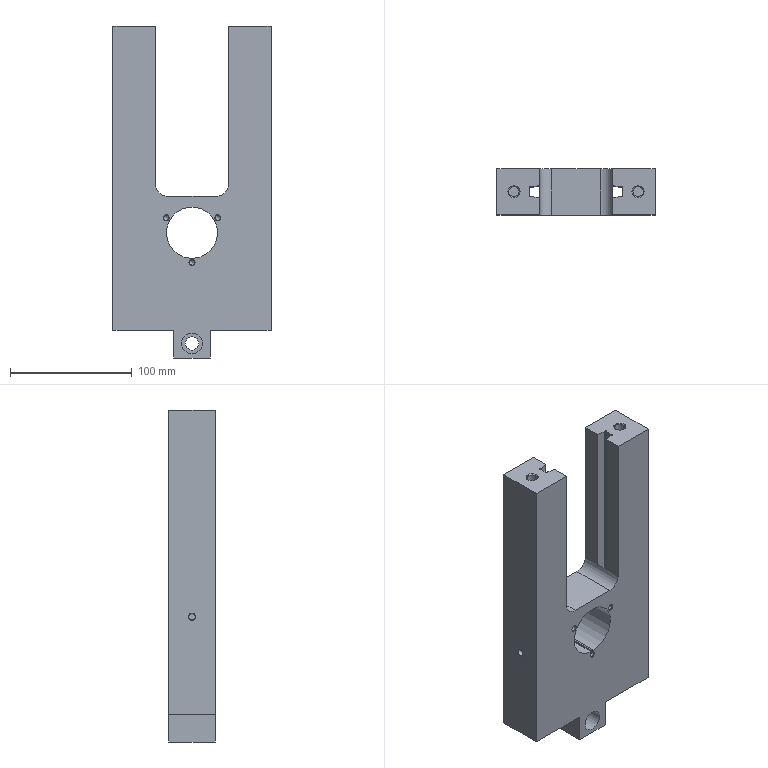Part | STEP file | YBQDJ-YB-6 | 1 solid | 72 faces | box 130 x 38 x 273 mm | volume 843391 mm3 | plane 31 | cylinder 29 | cone 12 | commonest cylinder face diameters 4 x10 1 x5 8.5 x4 4.2 x3 5.2 x2 20 x2